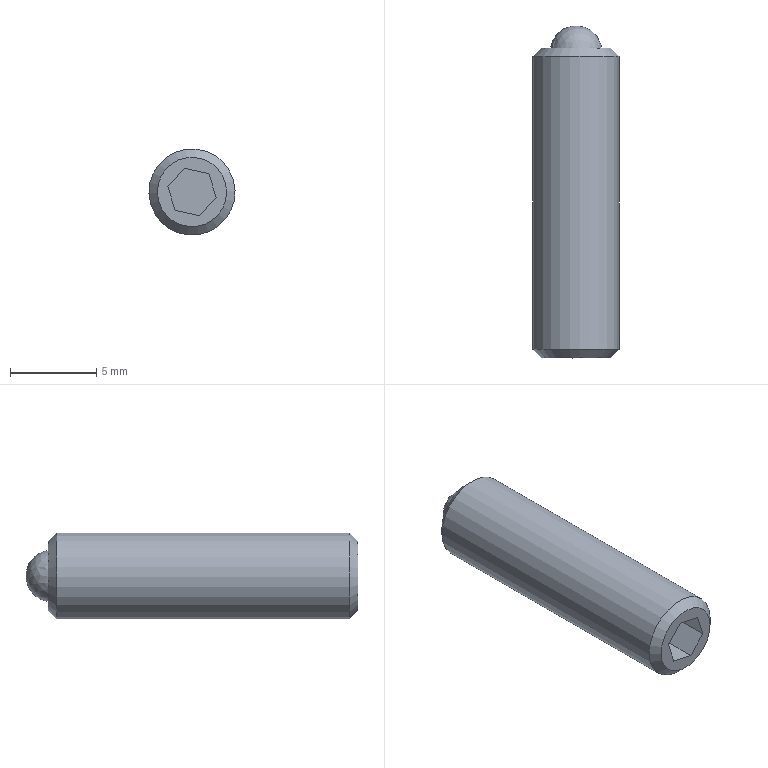Part | NX | features _ZAH04-M5 2 | 1 solid | 13 faces | box 5 x 19.3 x 5 mm | volume 344.732 mm3 | plane 9 | cone 2 | cylinder 1 | sphere 1 | commonest cylinder face diameters 5 x1
STEP:
#1=CARTESIAN_POINT('',(-32.557,55.49,-102.033));
#2=VERTEX_POINT('',#1);
#3=CARTESIAN_POINT('',(-35.,55.49,-101.5));
#4=DIRECTION('',(0.,1.,0.));
#5=DIRECTION('',(0.977,0.,-0.2131));
#6=AXIS2_PLACEMENT_3D('',#3,#4,#5);
#7=CIRCLE('',#6,2.5);
#8=EDGE_CURVE('',#2,#2,#7,.T.);
#9=ORIENTED_EDGE('',*,*,#8,.T.);
#10=EDGE_LOOP('',(#9));
#11=FACE_BOUND('',#10,.T.);
#12=CARTESIAN_POINT('',(-32.557,72.51,-102.033));
#13=VERTEX_POINT('',#12);
#14=CARTESIAN_POINT('',(-35.,72.51,-101.5));
#15=DIRECTION('',(0.,-1.,0.));
#16=DIRECTION('',(0.977,0.,-0.2131));
#17=AXIS2_PLACEMENT_3D('',#14,#15,#16);
#18=CIRCLE('',#17,2.5);
#19=EDGE_CURVE('',#13,#13,#18,.T.);
#20=ORIENTED_EDGE('',*,*,#19,.T.);
#21=EDGE_LOOP('',(#20));
#22=FACE_BOUND('',#21,.T.);
#23=CARTESIAN_POINT('',(-35.,73.,-101.5));
#24=DIRECTION('',(0.,-1.,0.));
#25=DIRECTION('',(-0.977,0.,0.2131));
#26=AXIS2_PLACEMENT_3D('',#23,#24,#25);
#27=CYLINDRICAL_SURFACE('',#26,2.5);
#28=ADVANCED_FACE('',(#11,#22),#27,.T.);
#29=ORIENTED_EDGE('',*,*,#8,.F.);
#30=EDGE_LOOP('',(#29));
#31=FACE_BOUND('',#30,.T.);
#32=CARTESIAN_POINT('',(-36.963,55.,-101.072));
#33=VERTEX_POINT('',#32);
#34=CARTESIAN_POINT('',(-35.,55.,-101.5));
#35=DIRECTION('',(0.,1.,0.));
#36=DIRECTION('',(-0.977,0.,0.2131));
#37=AXIS2_PLACEMENT_3D('',#34,#35,#36);
#38=CIRCLE('',#37,2.01);
#39=EDGE_CURVE('',#33,#33,#38,.T.);
#40=ORIENTED_EDGE('',*,*,#39,.T.);
#41=EDGE_LOOP('',(#40));
#42=FACE_BOUND('',#41,.T.);
#43=CARTESIAN_POINT('',(-35.,55.49,-101.5));
#44=DIRECTION('',(0.,1.,0.));
#45=DIRECTION('',(0.977,0.,-0.2131));
#46=AXIS2_PLACEMENT_3D('',#43,#44,#45);
#47=CONICAL_SURFACE('',#46,2.5,0.7854);
#48=ADVANCED_FACE('',(#31,#42),#47,.T.);
#49=ORIENTED_EDGE('',*,*,#19,.F.);
#50=EDGE_LOOP('',(#49));
#51=FACE_BOUND('',#50,.T.);
#52=CARTESIAN_POINT('',(-33.037,73.,-101.928));
#53=VERTEX_POINT('',#52);
#54=CARTESIAN_POINT('',(-35.,73.,-101.5));
#55=DIRECTION('',(0.,-1.,0.));
#56=DIRECTION('',(0.977,0.,-0.2131));
#57=AXIS2_PLACEMENT_3D('',#54,#55,#56);
#58=CIRCLE('',#57,2.009);
#59=EDGE_CURVE('',#53,#53,#58,.T.);
#60=ORIENTED_EDGE('',*,*,#59,.T.);
#61=EDGE_LOOP('',(#60));
#62=FACE_BOUND('',#61,.T.);
#63=CARTESIAN_POINT('',(-35.,72.509,-101.5));
#64=DIRECTION('',(0.,-1.,0.));
#65=DIRECTION('',(-0.977,0.,0.2131));
#66=AXIS2_PLACEMENT_3D('',#63,#64,#65);
#67=CONICAL_SURFACE('',#66,2.5,0.7854);
#68=ADVANCED_FACE('',(#51,#62),#67,.T.);
#69=CARTESIAN_POINT('',(-36.41,55.,-101.192));
#70=VERTEX_POINT('',#69);
#71=CARTESIAN_POINT('',(-35.439,55.,-100.125));
#72=VERTEX_POINT('',#71);
#73=CARTESIAN_POINT('',(-35.439,55.,-100.125));
#74=DIRECTION('',(0.6731,0.,0.7396));
#75=VECTOR('',#74,1000.);
#76=LINE('',#73,#75);
#77=EDGE_CURVE('',#70,#72,#76,.T.);
#78=ORIENTED_EDGE('',*,*,#77,.T.);
#79=CARTESIAN_POINT('',(-34.028,55.,-100.433));
#80=VERTEX_POINT('',#79);
#81=CARTESIAN_POINT('',(-34.028,55.,-100.433));
#82=DIRECTION('',(0.977,0.,-0.2131));
#83=VECTOR('',#82,1000.);
#84=LINE('',#81,#83);
#85=EDGE_CURVE('',#72,#80,#84,.T.);
#86=ORIENTED_EDGE('',*,*,#85,.T.);
#87=CARTESIAN_POINT('',(-33.59,55.,-101.808));
#88=VERTEX_POINT('',#87);
#89=CARTESIAN_POINT('',(-33.59,55.,-101.808));
#90=DIRECTION('',(0.3039,0.,-0.9527));
#91=VECTOR('',#90,1000.);
#92=LINE('',#89,#91);
#93=EDGE_CURVE('',#80,#88,#92,.T.);
#94=ORIENTED_EDGE('',*,*,#93,.T.);
#95=CARTESIAN_POINT('',(-34.561,55.,-102.875));
#96=VERTEX_POINT('',#95);
#97=CARTESIAN_POINT('',(-34.561,55.,-102.875));
#98=DIRECTION('',(-0.6731,0.,-0.7396));
#99=VECTOR('',#98,1000.);
#100=LINE('',#97,#99);
#101=EDGE_CURVE('',#88,#96,#100,.T.);
#102=ORIENTED_EDGE('',*,*,#101,.T.);
#103=CARTESIAN_POINT('',(-35.972,55.,-102.567));
#104=VERTEX_POINT('',#103);
#105=CARTESIAN_POINT('',(-35.972,55.,-102.567));
#106=DIRECTION('',(-0.977,0.,0.2131));
#107=VECTOR('',#106,1000.);
#108=LINE('',#105,#107);
#109=EDGE_CURVE('',#96,#104,#108,.T.);
#110=ORIENTED_EDGE('',*,*,#109,.T.);
#111=CARTESIAN_POINT('',(-36.41,55.,-101.192));
#112=DIRECTION('',(0.3039,0.,-0.9527));
#113=VECTOR('',#112,1000.);
#114=LINE('',#111,#113);
#115=EDGE_CURVE('',#70,#104,#114,.T.);
#116=ORIENTED_EDGE('',*,*,#115,.F.);
#117=EDGE_LOOP('',(#78,#86,#94,#102,#110,#116));
#118=FACE_BOUND('',#117,.T.);
#119=ORIENTED_EDGE('',*,*,#39,.F.);
#120=EDGE_LOOP('',(#119));
#121=FACE_BOUND('',#120,.T.);
#122=CARTESIAN_POINT('',(-35.,55.,-101.5));
#123=DIRECTION('',(0.,1.,0.));
#124=DIRECTION('',(0.977,0.,-0.2131));
#125=AXIS2_PLACEMENT_3D('',#122,#123,#124);
#126=PLANE('',#125);
#127=ADVANCED_FACE('',(#118,#121),#126,.F.);
#128=ORIENTED_EDGE('',*,*,#59,.F.);
#129=EDGE_LOOP('',(#128));
#130=FACE_BOUND('',#129,.T.);
#131=CARTESIAN_POINT('',(-33.548,73.,-101.817));
#132=VERTEX_POINT('',#131);
#133=CARTESIAN_POINT('',(-35.,73.,-101.5));
#134=DIRECTION('',(0.,-1.,0.));
#135=DIRECTION('',(0.977,0.,-0.2131));
#136=AXIS2_PLACEMENT_3D('',#133,#134,#135);
#137=CIRCLE('',#136,1.487);
#138=EDGE_CURVE('',#132,#132,#137,.F.);
#139=ORIENTED_EDGE('',*,*,#138,.F.);
#140=EDGE_LOOP('',(#139));
#141=FACE_BOUND('',#140,.T.);
#142=CARTESIAN_POINT('',(-35.428,73.,-103.463));
#143=DIRECTION('',(0.,-1.,0.));
#144=DIRECTION('',(-0.977,0.,0.2131));
#145=AXIS2_PLACEMENT_3D('',#142,#143,#144);
#146=PLANE('',#145);
#147=ADVANCED_FACE('',(#130,#141),#146,.F.);
#148=CARTESIAN_POINT('',(-35.972,57.,-102.567));
#149=VERTEX_POINT('',#148);
#150=CARTESIAN_POINT('',(-35.972,57.,-102.567));
#151=DIRECTION('',(0.,-1.,0.));
#152=VECTOR('',#151,1000.);
#153=LINE('',#150,#152);
#154=EDGE_CURVE('',#149,#104,#153,.T.);
#155=ORIENTED_EDGE('',*,*,#154,.F.);
#156=CARTESIAN_POINT('',(-36.41,57.,-101.192));
#157=VERTEX_POINT('',#156);
#158=CARTESIAN_POINT('',(-36.41,57.,-101.192));
#159=DIRECTION('',(0.3039,0.,-0.9527));
#160=VECTOR('',#159,1000.);
#161=LINE('',#158,#160);
#162=EDGE_CURVE('',#157,#149,#161,.T.);
#163=ORIENTED_EDGE('',*,*,#162,.F.);
#164=CARTESIAN_POINT('',(-36.41,57.,-101.192));
#165=DIRECTION('',(0.,1.,0.));
#166=VECTOR('',#165,1000.);
#167=LINE('',#164,#166);
#168=EDGE_CURVE('',#70,#157,#167,.T.);
#169=ORIENTED_EDGE('',*,*,#168,.F.);
#170=ORIENTED_EDGE('',*,*,#115,.T.);
#171=EDGE_LOOP('',(#155,#163,#169,#170));
#172=FACE_BOUND('',#171,.T.);
#173=CARTESIAN_POINT('',(-36.41,57.,-101.192));
#174=DIRECTION('',(-0.9527,0.,-0.3039));
#175=DIRECTION('',(0.3039,0.,-0.9527));
#176=AXIS2_PLACEMENT_3D('',#173,#174,#175);
#177=PLANE('',#176);
#178=ADVANCED_FACE('',(#172),#177,.F.);
#179=ORIENTED_EDGE('',*,*,#138,.T.);
#180=EDGE_LOOP('',(#179));
#181=FACE_BOUND('',#180,.T.);
#182=CARTESIAN_POINT('',(-35.,72.8,-101.5));
#183=DIRECTION('',(0.2131,0.,0.977));
#184=DIRECTION('',(0.9705,0.1154,-0.2117));
#185=AXIS2_PLACEMENT_3D('',#182,#183,#184);
#186=SPHERICAL_SURFACE('',#185,1.5);
#187=ADVANCED_FACE('',(#181),#186,.T.);
#188=ORIENTED_EDGE('',*,*,#109,.F.);
#189=CARTESIAN_POINT('',(-34.561,57.,-102.875));
#190=VERTEX_POINT('',#189);
#191=CARTESIAN_POINT('',(-34.561,57.,-102.875));
#192=DIRECTION('',(0.,-1.,0.));
#193=VECTOR('',#192,1000.);
#194=LINE('',#191,#193);
#195=EDGE_CURVE('',#190,#96,#194,.T.);
#196=ORIENTED_EDGE('',*,*,#195,.F.);
#197=CARTESIAN_POINT('',(-35.972,57.,-102.567));
#198=DIRECTION('',(0.977,0.,-0.2131));
#199=VECTOR('',#198,1000.);
#200=LINE('',#197,#199);
#201=EDGE_CURVE('',#149,#190,#200,.T.);
#202=ORIENTED_EDGE('',*,*,#201,.F.);
#203=ORIENTED_EDGE('',*,*,#154,.T.);
#204=EDGE_LOOP('',(#188,#196,#202,#203));
#205=FACE_BOUND('',#204,.T.);
#206=CARTESIAN_POINT('',(-35.972,57.,-102.567));
#207=DIRECTION('',(-0.2131,0.,-0.977));
#208=DIRECTION('',(0.,1.,0.));
#209=AXIS2_PLACEMENT_3D('',#206,#207,#208);
#210=PLANE('',#209);
#211=ADVANCED_FACE('',(#205),#210,.F.);
#212=CARTESIAN_POINT('',(-33.59,57.,-101.808));
#213=VERTEX_POINT('',#212);
#214=CARTESIAN_POINT('',(-34.561,57.,-102.875));
#215=DIRECTION('',(0.6731,0.,0.7396));
#216=VECTOR('',#215,1000.);
#217=LINE('',#214,#216);
#218=EDGE_CURVE('',#190,#213,#217,.T.);
#219=ORIENTED_EDGE('',*,*,#218,.T.);
#220=CARTESIAN_POINT('',(-34.028,57.,-100.433));
#221=VERTEX_POINT('',#220);
#222=CARTESIAN_POINT('',(-33.59,57.,-101.808));
#223=DIRECTION('',(-0.3039,0.,0.9527));
#224=VECTOR('',#223,1000.);
#225=LINE('',#222,#224);
#226=EDGE_CURVE('',#213,#221,#225,.T.);
#227=ORIENTED_EDGE('',*,*,#226,.T.);
#228=CARTESIAN_POINT('',(-35.439,57.,-100.125));
#229=VERTEX_POINT('',#228);
#230=CARTESIAN_POINT('',(-34.028,57.,-100.433));
#231=DIRECTION('',(-0.977,0.,0.2131));
#232=VECTOR('',#231,1000.);
#233=LINE('',#230,#232);
#234=EDGE_CURVE('',#221,#229,#233,.T.);
#235=ORIENTED_EDGE('',*,*,#234,.T.);
#236=CARTESIAN_POINT('',(-35.439,57.,-100.125));
#237=DIRECTION('',(-0.6731,0.,-0.7396));
#238=VECTOR('',#237,1000.);
#239=LINE('',#236,#238);
#240=EDGE_CURVE('',#229,#157,#239,.T.);
#241=ORIENTED_EDGE('',*,*,#240,.T.);
#242=ORIENTED_EDGE('',*,*,#162,.T.);
#243=ORIENTED_EDGE('',*,*,#201,.T.);
#244=EDGE_LOOP('',(#219,#227,#235,#241,#242,#243));
#245=FACE_BOUND('',#244,.T.);
#246=CARTESIAN_POINT('',(-35.,57.,-101.5));
#247=DIRECTION('',(0.,-1.,0.));
#248=DIRECTION('',(-0.977,0.,0.2131));
#249=AXIS2_PLACEMENT_3D('',#246,#247,#248);
#250=PLANE('',#249);
#251=ADVANCED_FACE('',(#245),#250,.T.);
#252=ORIENTED_EDGE('',*,*,#168,.T.);
#253=ORIENTED_EDGE('',*,*,#240,.F.);
#254=CARTESIAN_POINT('',(-35.439,57.,-100.125));
#255=DIRECTION('',(0.,1.,0.));
#256=VECTOR('',#255,1000.);
#257=LINE('',#254,#256);
#258=EDGE_CURVE('',#72,#229,#257,.T.);
#259=ORIENTED_EDGE('',*,*,#258,.F.);
#260=ORIENTED_EDGE('',*,*,#77,.F.);
#261=EDGE_LOOP('',(#252,#253,#259,#260));
#262=FACE_BOUND('',#261,.T.);
#263=CARTESIAN_POINT('',(-35.439,57.,-100.125));
#264=DIRECTION('',(-0.7396,0.,0.6731));
#265=DIRECTION('',(-0.6731,0.,-0.7396));
#266=AXIS2_PLACEMENT_3D('',#263,#264,#265);
#267=PLANE('',#266);
#268=ADVANCED_FACE('',(#262),#267,.F.);
#269=CARTESIAN_POINT('',(-33.59,57.,-101.808));
#270=DIRECTION('',(0.,-1.,0.));
#271=VECTOR('',#270,1000.);
#272=LINE('',#269,#271);
#273=EDGE_CURVE('',#213,#88,#272,.T.);
#274=ORIENTED_EDGE('',*,*,#273,.F.);
#275=ORIENTED_EDGE('',*,*,#218,.F.);
#276=ORIENTED_EDGE('',*,*,#195,.T.);
#277=ORIENTED_EDGE('',*,*,#101,.F.);
#278=EDGE_LOOP('',(#274,#275,#276,#277));
#279=FACE_BOUND('',#278,.T.);
#280=CARTESIAN_POINT('',(-34.561,57.,-102.875));
#281=DIRECTION('',(0.7396,0.,-0.6731));
#282=DIRECTION('',(0.6731,0.,0.7396));
#283=AXIS2_PLACEMENT_3D('',#280,#281,#282);
#284=PLANE('',#283);
#285=ADVANCED_FACE('',(#279),#284,.F.);
#286=ORIENTED_EDGE('',*,*,#258,.T.);
#287=ORIENTED_EDGE('',*,*,#234,.F.);
#288=CARTESIAN_POINT('',(-34.028,57.,-100.433));
#289=DIRECTION('',(0.,1.,0.));
#290=VECTOR('',#289,1000.);
#291=LINE('',#288,#290);
#292=EDGE_CURVE('',#80,#221,#291,.T.);
#293=ORIENTED_EDGE('',*,*,#292,.F.);
#294=ORIENTED_EDGE('',*,*,#85,.F.);
#295=EDGE_LOOP('',(#286,#287,#293,#294));
#296=FACE_BOUND('',#295,.T.);
#297=CARTESIAN_POINT('',(-34.028,57.,-100.433));
#298=DIRECTION('',(0.2131,0.,0.977));
#299=DIRECTION('',(0.,-1.,0.));
#300=AXIS2_PLACEMENT_3D('',#297,#298,#299);
#301=PLANE('',#300);
#302=ADVANCED_FACE('',(#296),#301,.F.);
#303=ORIENTED_EDGE('',*,*,#292,.T.);
#304=ORIENTED_EDGE('',*,*,#226,.F.);
#305=ORIENTED_EDGE('',*,*,#273,.T.);
#306=ORIENTED_EDGE('',*,*,#93,.F.);
#307=EDGE_LOOP('',(#303,#304,#305,#306));
#308=FACE_BOUND('',#307,.T.);
#309=CARTESIAN_POINT('',(-33.59,57.,-101.808));
#310=DIRECTION('',(0.9527,0.,0.3039));
#311=DIRECTION('',(-0.3039,0.,0.9527));
#312=AXIS2_PLACEMENT_3D('',#309,#310,#311);
#313=PLANE('',#312);
#314=ADVANCED_FACE('',(#308),#313,.F.);
#315=CLOSED_SHELL('',(#28,#48,#68,#127,#147,#178,#187,#211,#251,#268,#285,#302,#314));
#316=MANIFOLD_SOLID_BREP('',#315);
#317=(LENGTH_UNIT()NAMED_UNIT(*)SI_UNIT(.MILLI.,.METRE.));
#318=UNCERTAINTY_MEASURE_WITH_UNIT(LENGTH_MEASURE(0.00001),#317,'','');
#319=(NAMED_UNIT(*)PLANE_ANGLE_UNIT()SI_UNIT($,.RADIAN.));
#320=(NAMED_UNIT(*)SI_UNIT($,.STERADIAN.)SOLID_ANGLE_UNIT());
#321=(GEOMETRIC_REPRESENTATION_CONTEXT(3)GLOBAL_UNCERTAINTY_ASSIGNED_CONTEXT((#318))GLOBAL_UNIT_ASSIGNED_CONTEXT((#317,#319,#320))REPRESENTATION_CONTEXT('',''));
#322=ADVANCED_BREP_SHAPE_REPRESENTATION('',(#316),#321);